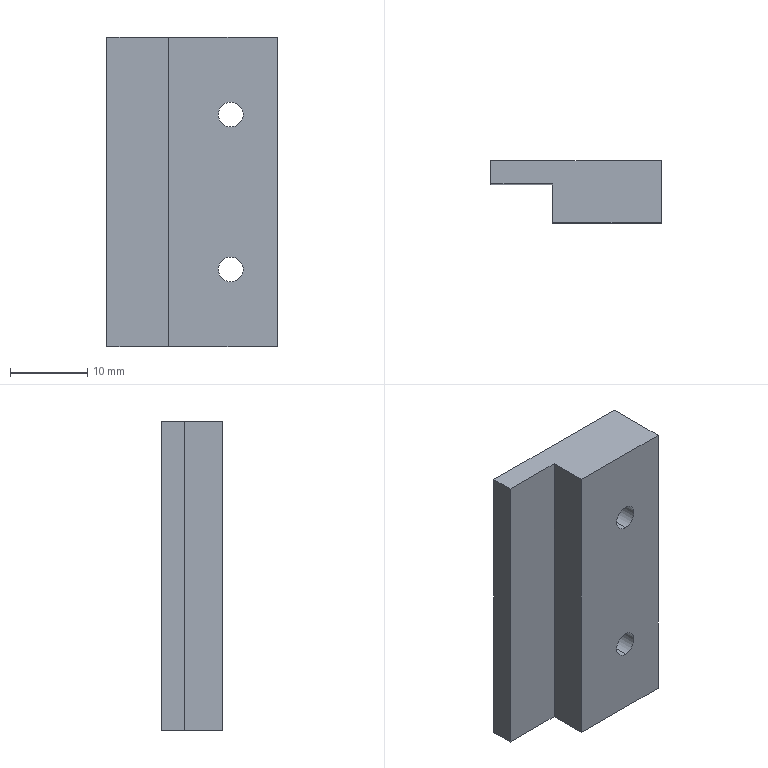Part | STEP file | PN_0053 | 1 solid | 12 faces | box 22 x 8 x 40 mm | volume 5311 mm3 | plane 8 | cylinder 4 | commonest cylinder face diameters 3.2 x4
STEP:
#1=CARTESIAN_POINT('',(0.,0.,0.));
#2=DIRECTION('',(0.,0.,1.));
#3=DIRECTION('',(1.,0.,0.));
#4=AXIS2_PLACEMENT_3D('',#1,#2,#3);
#5=CARTESIAN_POINT('',(5.,0.,11.6));
#6=VERTEX_POINT('',#5);
#7=CARTESIAN_POINT('',(5.,8.,11.6));
#8=VERTEX_POINT('',#7);
#9=CARTESIAN_POINT('',(5.,8.,11.6));
#10=DIRECTION('',(0.,1.,0.));
#11=VECTOR('',#10,1.);
#12=LINE('',#9,#11);
#13=CARTESIAN_POINT('',(5.,8.,10.));
#14=DIRECTION('',(0.,1.,0.));
#15=DIRECTION('',(0.,0.,1.));
#16=AXIS2_PLACEMENT_3D('',#13,#14,#15);
#17=CYLINDRICAL_SURFACE('',#16,1.6);
#18=CARTESIAN_POINT('',(6.283,0.));
#19=DIRECTION('',(0.,1.));
#20=VECTOR('',#19,1.);
#21=LINE('',#18,#20);
#22=(GEOMETRIC_REPRESENTATION_CONTEXT(2)PARAMETRIC_REPRESENTATION_CONTEXT()REPRESENTATION_CONTEXT('',''));
#23=DEFINITIONAL_REPRESENTATION('',(#21),#22);
#24=PCURVE('',#17,#23);
#25=CARTESIAN_POINT('',(5.,8.,10.));
#26=DIRECTION('',(0.,1.,0.));
#27=DIRECTION('',(0.,0.,1.));
#28=AXIS2_PLACEMENT_3D('',#25,#26,#27);
#29=CYLINDRICAL_SURFACE('',#28,1.6);
#30=CARTESIAN_POINT('',(0.,0.));
#31=DIRECTION('',(0.,1.));
#32=VECTOR('',#31,1.);
#33=LINE('',#30,#32);
#34=(GEOMETRIC_REPRESENTATION_CONTEXT(2)PARAMETRIC_REPRESENTATION_CONTEXT()REPRESENTATION_CONTEXT('',''));
#35=DEFINITIONAL_REPRESENTATION('',(#33),#34);
#36=PCURVE('',#29,#35);
#37=SURFACE_CURVE('',#12,(#24,#36),.PCURVE_S1.);
#38=EDGE_CURVE('',#6,#8,#37,.T.);
#39=ORIENTED_EDGE('',*,*,#38,.T.);
#40=CARTESIAN_POINT('',(5.,8.,8.4));
#41=VERTEX_POINT('',#40);
#42=CARTESIAN_POINT('',(5.,8.,10.));
#43=DIRECTION('',(0.,1.,0.));
#44=DIRECTION('',(0.,0.,1.));
#45=AXIS2_PLACEMENT_3D('',#42,#43,#44);
#46=CIRCLE('',#45,1.6);
#47=CARTESIAN_POINT('',(0.,0.));
#48=DIRECTION('',(1.,0.));
#49=VECTOR('',#48,1.);
#50=LINE('',#47,#49);
#51=(GEOMETRIC_REPRESENTATION_CONTEXT(2)PARAMETRIC_REPRESENTATION_CONTEXT()REPRESENTATION_CONTEXT('',''));
#52=DEFINITIONAL_REPRESENTATION('',(#50),#51);
#53=PCURVE('',#17,#52);
#54=CARTESIAN_POINT('',(0.,8.,0.));
#55=DIRECTION('',(0.,1.,0.));
#56=DIRECTION('',(0.,0.,1.));
#57=AXIS2_PLACEMENT_3D('',#54,#55,#56);
#58=PLANE('',#57);
#59=CARTESIAN_POINT('',(10.,5.));
#60=DIRECTION('',(1.,0.));
#61=AXIS2_PLACEMENT_2D('',#59,#60);
#62=CIRCLE('',#61,1.6);
#63=(GEOMETRIC_REPRESENTATION_CONTEXT(2)PARAMETRIC_REPRESENTATION_CONTEXT()REPRESENTATION_CONTEXT('',''));
#64=DEFINITIONAL_REPRESENTATION('',(#62),#63);
#65=PCURVE('',#58,#64);
#66=SURFACE_CURVE('',#46,(#53,#65),.PCURVE_S1.);
#67=EDGE_CURVE('',#41,#8,#66,.T.);
#68=ORIENTED_EDGE('',*,*,#67,.F.);
#69=CARTESIAN_POINT('',(5.,0.,8.4));
#70=VERTEX_POINT('',#69);
#71=CARTESIAN_POINT('',(5.,8.,8.4));
#72=DIRECTION('',(0.,1.,0.));
#73=VECTOR('',#72,1.);
#74=LINE('',#71,#73);
#75=CARTESIAN_POINT('',(3.142,0.));
#76=DIRECTION('',(0.,1.));
#77=VECTOR('',#76,1.);
#78=LINE('',#75,#77);
#79=(GEOMETRIC_REPRESENTATION_CONTEXT(2)PARAMETRIC_REPRESENTATION_CONTEXT()REPRESENTATION_CONTEXT('',''));
#80=DEFINITIONAL_REPRESENTATION('',(#78),#79);
#81=PCURVE('',#17,#80);
#82=CARTESIAN_POINT('',(3.142,0.));
#83=DIRECTION('',(0.,1.));
#84=VECTOR('',#83,1.);
#85=LINE('',#82,#84);
#86=(GEOMETRIC_REPRESENTATION_CONTEXT(2)PARAMETRIC_REPRESENTATION_CONTEXT()REPRESENTATION_CONTEXT('',''));
#87=DEFINITIONAL_REPRESENTATION('',(#85),#86);
#88=PCURVE('',#29,#87);
#89=SURFACE_CURVE('',#74,(#81,#88),.PCURVE_S1.);
#90=EDGE_CURVE('',#70,#41,#89,.T.);
#91=ORIENTED_EDGE('',*,*,#90,.F.);
#92=CARTESIAN_POINT('',(5.,0.,10.));
#93=DIRECTION('',(0.,1.,0.));
#94=DIRECTION('',(0.,0.,1.));
#95=AXIS2_PLACEMENT_3D('',#92,#93,#94);
#96=CIRCLE('',#95,1.6);
#97=CARTESIAN_POINT('',(0.,-8.));
#98=DIRECTION('',(1.,0.));
#99=VECTOR('',#98,1.);
#100=LINE('',#97,#99);
#101=(GEOMETRIC_REPRESENTATION_CONTEXT(2)PARAMETRIC_REPRESENTATION_CONTEXT()REPRESENTATION_CONTEXT('',''));
#102=DEFINITIONAL_REPRESENTATION('',(#100),#101);
#103=PCURVE('',#17,#102);
#104=CARTESIAN_POINT('',(0.,0.,0.));
#105=DIRECTION('',(0.,1.,0.));
#106=DIRECTION('',(0.,0.,1.));
#107=AXIS2_PLACEMENT_3D('',#104,#105,#106);
#108=PLANE('',#107);
#109=CARTESIAN_POINT('',(10.,5.));
#110=DIRECTION('',(1.,0.));
#111=AXIS2_PLACEMENT_2D('',#109,#110);
#112=CIRCLE('',#111,1.6);
#113=(GEOMETRIC_REPRESENTATION_CONTEXT(2)PARAMETRIC_REPRESENTATION_CONTEXT()REPRESENTATION_CONTEXT('',''));
#114=DEFINITIONAL_REPRESENTATION('',(#112),#113);
#115=PCURVE('',#108,#114);
#116=SURFACE_CURVE('',#96,(#103,#115),.PCURVE_S1.);
#117=EDGE_CURVE('',#70,#6,#116,.T.);
#118=ORIENTED_EDGE('',*,*,#117,.T.);
#119=EDGE_LOOP('',(#39,#68,#91,#118));
#120=FACE_BOUND('',#119,.F.);
#121=ADVANCED_FACE('',(#120),#17,.F.);
#122=CARTESIAN_POINT('',(5.,0.,-8.4));
#123=VERTEX_POINT('',#122);
#124=CARTESIAN_POINT('',(5.,8.,-8.4));
#125=VERTEX_POINT('',#124);
#126=CARTESIAN_POINT('',(5.,8.,-8.4));
#127=DIRECTION('',(0.,1.,0.));
#128=VECTOR('',#127,1.);
#129=LINE('',#126,#128);
#130=CARTESIAN_POINT('',(5.,8.,-10.));
#131=DIRECTION('',(0.,1.,0.));
#132=DIRECTION('',(0.,0.,1.));
#133=AXIS2_PLACEMENT_3D('',#130,#131,#132);
#134=CYLINDRICAL_SURFACE('',#133,1.6);
#135=CARTESIAN_POINT('',(6.283,0.));
#136=DIRECTION('',(0.,1.));
#137=VECTOR('',#136,1.);
#138=LINE('',#135,#137);
#139=(GEOMETRIC_REPRESENTATION_CONTEXT(2)PARAMETRIC_REPRESENTATION_CONTEXT()REPRESENTATION_CONTEXT('',''));
#140=DEFINITIONAL_REPRESENTATION('',(#138),#139);
#141=PCURVE('',#134,#140);
#142=CARTESIAN_POINT('',(5.,8.,-10.));
#143=DIRECTION('',(0.,1.,0.));
#144=DIRECTION('',(0.,0.,1.));
#145=AXIS2_PLACEMENT_3D('',#142,#143,#144);
#146=CYLINDRICAL_SURFACE('',#145,1.6);
#147=CARTESIAN_POINT('',(0.,0.));
#148=DIRECTION('',(0.,1.));
#149=VECTOR('',#148,1.);
#150=LINE('',#147,#149);
#151=(GEOMETRIC_REPRESENTATION_CONTEXT(2)PARAMETRIC_REPRESENTATION_CONTEXT()REPRESENTATION_CONTEXT('',''));
#152=DEFINITIONAL_REPRESENTATION('',(#150),#151);
#153=PCURVE('',#146,#152);
#154=SURFACE_CURVE('',#129,(#141,#153),.PCURVE_S1.);
#155=EDGE_CURVE('',#123,#125,#154,.T.);
#156=ORIENTED_EDGE('',*,*,#155,.T.);
#157=CARTESIAN_POINT('',(5.,8.,-11.6));
#158=VERTEX_POINT('',#157);
#159=CARTESIAN_POINT('',(5.,8.,-10.));
#160=DIRECTION('',(0.,1.,0.));
#161=DIRECTION('',(0.,0.,1.));
#162=AXIS2_PLACEMENT_3D('',#159,#160,#161);
#163=CIRCLE('',#162,1.6);
#164=CARTESIAN_POINT('',(0.,0.));
#165=DIRECTION('',(1.,0.));
#166=VECTOR('',#165,1.);
#167=LINE('',#164,#166);
#168=(GEOMETRIC_REPRESENTATION_CONTEXT(2)PARAMETRIC_REPRESENTATION_CONTEXT()REPRESENTATION_CONTEXT('',''));
#169=DEFINITIONAL_REPRESENTATION('',(#167),#168);
#170=PCURVE('',#134,#169);
#171=CARTESIAN_POINT('',(-10.,5.));
#172=DIRECTION('',(1.,0.));
#173=AXIS2_PLACEMENT_2D('',#171,#172);
#174=CIRCLE('',#173,1.6);
#175=(GEOMETRIC_REPRESENTATION_CONTEXT(2)PARAMETRIC_REPRESENTATION_CONTEXT()REPRESENTATION_CONTEXT('',''));
#176=DEFINITIONAL_REPRESENTATION('',(#174),#175);
#177=PCURVE('',#58,#176);
#178=SURFACE_CURVE('',#163,(#170,#177),.PCURVE_S1.);
#179=EDGE_CURVE('',#158,#125,#178,.T.);
#180=ORIENTED_EDGE('',*,*,#179,.F.);
#181=CARTESIAN_POINT('',(5.,0.,-11.6));
#182=VERTEX_POINT('',#181);
#183=CARTESIAN_POINT('',(5.,8.,-11.6));
#184=DIRECTION('',(0.,1.,0.));
#185=VECTOR('',#184,1.);
#186=LINE('',#183,#185);
#187=CARTESIAN_POINT('',(3.142,0.));
#188=DIRECTION('',(0.,1.));
#189=VECTOR('',#188,1.);
#190=LINE('',#187,#189);
#191=(GEOMETRIC_REPRESENTATION_CONTEXT(2)PARAMETRIC_REPRESENTATION_CONTEXT()REPRESENTATION_CONTEXT('',''));
#192=DEFINITIONAL_REPRESENTATION('',(#190),#191);
#193=PCURVE('',#134,#192);
#194=CARTESIAN_POINT('',(3.142,0.));
#195=DIRECTION('',(0.,1.));
#196=VECTOR('',#195,1.);
#197=LINE('',#194,#196);
#198=(GEOMETRIC_REPRESENTATION_CONTEXT(2)PARAMETRIC_REPRESENTATION_CONTEXT()REPRESENTATION_CONTEXT('',''));
#199=DEFINITIONAL_REPRESENTATION('',(#197),#198);
#200=PCURVE('',#146,#199);
#201=SURFACE_CURVE('',#186,(#193,#200),.PCURVE_S1.);
#202=EDGE_CURVE('',#182,#158,#201,.T.);
#203=ORIENTED_EDGE('',*,*,#202,.F.);
#204=CARTESIAN_POINT('',(5.,0.,-10.));
#205=DIRECTION('',(0.,1.,0.));
#206=DIRECTION('',(0.,0.,1.));
#207=AXIS2_PLACEMENT_3D('',#204,#205,#206);
#208=CIRCLE('',#207,1.6);
#209=CARTESIAN_POINT('',(0.,-8.));
#210=DIRECTION('',(1.,0.));
#211=VECTOR('',#210,1.);
#212=LINE('',#209,#211);
#213=(GEOMETRIC_REPRESENTATION_CONTEXT(2)PARAMETRIC_REPRESENTATION_CONTEXT()REPRESENTATION_CONTEXT('',''));
#214=DEFINITIONAL_REPRESENTATION('',(#212),#213);
#215=PCURVE('',#134,#214);
#216=CARTESIAN_POINT('',(-10.,5.));
#217=DIRECTION('',(1.,0.));
#218=AXIS2_PLACEMENT_2D('',#216,#217);
#219=CIRCLE('',#218,1.6);
#220=(GEOMETRIC_REPRESENTATION_CONTEXT(2)PARAMETRIC_REPRESENTATION_CONTEXT()REPRESENTATION_CONTEXT('',''));
#221=DEFINITIONAL_REPRESENTATION('',(#219),#220);
#222=PCURVE('',#108,#221);
#223=SURFACE_CURVE('',#208,(#215,#222),.PCURVE_S1.);
#224=EDGE_CURVE('',#182,#123,#223,.T.);
#225=ORIENTED_EDGE('',*,*,#224,.T.);
#226=EDGE_LOOP('',(#156,#180,#203,#225));
#227=FACE_BOUND('',#226,.F.);
#228=ADVANCED_FACE('',(#227),#134,.F.);
#229=CARTESIAN_POINT('',(11.,0.,20.));
#230=VERTEX_POINT('',#229);
#231=CARTESIAN_POINT('',(11.,0.,-20.));
#232=VERTEX_POINT('',#231);
#233=CARTESIAN_POINT('',(11.,0.,-20.));
#234=DIRECTION('',(0.,0.,-1.));
#235=VECTOR('',#234,1.);
#236=LINE('',#233,#235);
#237=CARTESIAN_POINT('',(11.,8.,-20.));
#238=DIRECTION('',(-1.,0.,0.));
#239=DIRECTION('',(0.,0.,1.));
#240=AXIS2_PLACEMENT_3D('',#237,#238,#239);
#241=PLANE('',#240);
#242=CARTESIAN_POINT('',(0.,-8.));
#243=DIRECTION('',(-1.,0.));
#244=VECTOR('',#243,1.);
#245=LINE('',#242,#244);
#246=(GEOMETRIC_REPRESENTATION_CONTEXT(2)PARAMETRIC_REPRESENTATION_CONTEXT()REPRESENTATION_CONTEXT('',''));
#247=DEFINITIONAL_REPRESENTATION('',(#245),#246);
#248=PCURVE('',#241,#247);
#249=CARTESIAN_POINT('',(-20.,11.));
#250=DIRECTION('',(-1.,0.));
#251=VECTOR('',#250,1.);
#252=LINE('',#249,#251);
#253=(GEOMETRIC_REPRESENTATION_CONTEXT(2)PARAMETRIC_REPRESENTATION_CONTEXT()REPRESENTATION_CONTEXT('',''));
#254=DEFINITIONAL_REPRESENTATION('',(#252),#253);
#255=PCURVE('',#108,#254);
#256=SURFACE_CURVE('',#236,(#248,#255),.PCURVE_S1.);
#257=EDGE_CURVE('',#230,#232,#256,.T.);
#258=ORIENTED_EDGE('',*,*,#257,.T.);
#259=CARTESIAN_POINT('',(11.,8.,-20.));
#260=VERTEX_POINT('',#259);
#261=CARTESIAN_POINT('',(11.,8.,-20.));
#262=DIRECTION('',(0.,-1.,0.));
#263=VECTOR('',#262,1.);
#264=LINE('',#261,#263);
#265=CARTESIAN_POINT('',(0.,0.));
#266=DIRECTION('',(0.,-1.));
#267=VECTOR('',#266,1.);
#268=LINE('',#265,#267);
#269=(GEOMETRIC_REPRESENTATION_CONTEXT(2)PARAMETRIC_REPRESENTATION_CONTEXT()REPRESENTATION_CONTEXT('',''));
#270=DEFINITIONAL_REPRESENTATION('',(#268),#269);
#271=PCURVE('',#241,#270);
#272=CARTESIAN_POINT('',(-11.,8.,-20.));
#273=DIRECTION('',(0.,0.,1.));
#274=DIRECTION('',(1.,0.,0.));
#275=AXIS2_PLACEMENT_3D('',#272,#273,#274);
#276=PLANE('',#275);
#277=CARTESIAN_POINT('',(22.,0.));
#278=DIRECTION('',(0.,-1.));
#279=VECTOR('',#278,1.);
#280=LINE('',#277,#279);
#281=(GEOMETRIC_REPRESENTATION_CONTEXT(2)PARAMETRIC_REPRESENTATION_CONTEXT()REPRESENTATION_CONTEXT('',''));
#282=DEFINITIONAL_REPRESENTATION('',(#280),#281);
#283=PCURVE('',#276,#282);
#284=SURFACE_CURVE('',#264,(#271,#283),.PCURVE_S1.);
#285=EDGE_CURVE('',#260,#232,#284,.T.);
#286=ORIENTED_EDGE('',*,*,#285,.F.);
#287=CARTESIAN_POINT('',(11.,8.,20.));
#288=VERTEX_POINT('',#287);
#289=CARTESIAN_POINT('',(11.,8.,-20.));
#290=DIRECTION('',(0.,0.,-1.));
#291=VECTOR('',#290,1.);
#292=LINE('',#289,#291);
#293=CARTESIAN_POINT('',(0.,0.));
#294=DIRECTION('',(-1.,0.));
#295=VECTOR('',#294,1.);
#296=LINE('',#293,#295);
#297=(GEOMETRIC_REPRESENTATION_CONTEXT(2)PARAMETRIC_REPRESENTATION_CONTEXT()REPRESENTATION_CONTEXT('',''));
#298=DEFINITIONAL_REPRESENTATION('',(#296),#297);
#299=PCURVE('',#241,#298);
#300=CARTESIAN_POINT('',(-20.,11.));
#301=DIRECTION('',(-1.,0.));
#302=VECTOR('',#301,1.);
#303=LINE('',#300,#302);
#304=(GEOMETRIC_REPRESENTATION_CONTEXT(2)PARAMETRIC_REPRESENTATION_CONTEXT()REPRESENTATION_CONTEXT('',''));
#305=DEFINITIONAL_REPRESENTATION('',(#303),#304);
#306=PCURVE('',#58,#305);
#307=SURFACE_CURVE('',#292,(#299,#306),.PCURVE_S1.);
#308=EDGE_CURVE('',#288,#260,#307,.T.);
#309=ORIENTED_EDGE('',*,*,#308,.F.);
#310=CARTESIAN_POINT('',(11.,8.,20.));
#311=DIRECTION('',(0.,-1.,0.));
#312=VECTOR('',#311,1.);
#313=LINE('',#310,#312);
#314=CARTESIAN_POINT('',(40.,0.));
#315=DIRECTION('',(0.,-1.));
#316=VECTOR('',#315,1.);
#317=LINE('',#314,#316);
#318=(GEOMETRIC_REPRESENTATION_CONTEXT(2)PARAMETRIC_REPRESENTATION_CONTEXT()REPRESENTATION_CONTEXT('',''));
#319=DEFINITIONAL_REPRESENTATION('',(#317),#318);
#320=PCURVE('',#241,#319);
#321=CARTESIAN_POINT('',(-11.,8.,20.));
#322=DIRECTION('',(0.,0.,-1.));
#323=DIRECTION('',(-1.,0.,0.));
#324=AXIS2_PLACEMENT_3D('',#321,#322,#323);
#325=PLANE('',#324);
#326=CARTESIAN_POINT('',(-22.,0.));
#327=DIRECTION('',(0.,-1.));
#328=VECTOR('',#327,1.);
#329=LINE('',#326,#328);
#330=(GEOMETRIC_REPRESENTATION_CONTEXT(2)PARAMETRIC_REPRESENTATION_CONTEXT()REPRESENTATION_CONTEXT('',''));
#331=DEFINITIONAL_REPRESENTATION('',(#329),#330);
#332=PCURVE('',#325,#331);
#333=SURFACE_CURVE('',#313,(#320,#332),.PCURVE_S1.);
#334=EDGE_CURVE('',#288,#230,#333,.T.);
#335=ORIENTED_EDGE('',*,*,#334,.T.);
#336=EDGE_LOOP('',(#258,#286,#309,#335));
#337=FACE_BOUND('',#336,.T.);
#338=ADVANCED_FACE('',(#337),#241,.F.);
#339=CARTESIAN_POINT('',(-3.,0.,-20.));
#340=VERTEX_POINT('',#339);
#341=CARTESIAN_POINT('',(-3.,5.,-20.));
#342=VERTEX_POINT('',#341);
#343=CARTESIAN_POINT('',(-3.,0.,-20.));
#344=DIRECTION('',(0.,1.,0.));
#345=VECTOR('',#344,1.);
#346=LINE('',#343,#345);
#347=CARTESIAN_POINT('',(8.,-8.));
#348=DIRECTION('',(0.,1.));
#349=VECTOR('',#348,1.);
#350=LINE('',#347,#349);
#351=(GEOMETRIC_REPRESENTATION_CONTEXT(2)PARAMETRIC_REPRESENTATION_CONTEXT()REPRESENTATION_CONTEXT('',''));
#352=DEFINITIONAL_REPRESENTATION('',(#350),#351);
#353=PCURVE('',#276,#352);
#354=CARTESIAN_POINT('',(-3.,0.,-20.));
#355=DIRECTION('',(1.,0.,0.));
#356=DIRECTION('',(0.,0.,-1.));
#357=AXIS2_PLACEMENT_3D('',#354,#355,#356);
#358=PLANE('',#357);
#359=CARTESIAN_POINT('',(0.,0.));
#360=DIRECTION('',(0.,1.));
#361=VECTOR('',#360,1.);
#362=LINE('',#359,#361);
#363=(GEOMETRIC_REPRESENTATION_CONTEXT(2)PARAMETRIC_REPRESENTATION_CONTEXT()REPRESENTATION_CONTEXT('',''));
#364=DEFINITIONAL_REPRESENTATION('',(#362),#363);
#365=PCURVE('',#358,#364);
#366=SURFACE_CURVE('',#346,(#353,#365),.PCURVE_S1.);
#367=EDGE_CURVE('',#340,#342,#366,.T.);
#368=ORIENTED_EDGE('',*,*,#367,.T.);
#369=CARTESIAN_POINT('',(-11.,5.,-20.));
#370=VERTEX_POINT('',#369);
#371=CARTESIAN_POINT('',(-11.,5.,-20.));
#372=DIRECTION('',(-1.,0.,0.));
#373=VECTOR('',#372,1.);
#374=LINE('',#371,#373);
#375=CARTESIAN_POINT('',(0.,-3.));
#376=DIRECTION('',(-1.,0.));
#377=VECTOR('',#376,1.);
#378=LINE('',#375,#377);
#379=(GEOMETRIC_REPRESENTATION_CONTEXT(2)PARAMETRIC_REPRESENTATION_CONTEXT()REPRESENTATION_CONTEXT('',''));
#380=DEFINITIONAL_REPRESENTATION('',(#378),#379);
#381=PCURVE('',#276,#380);
#382=CARTESIAN_POINT('',(-11.,5.,-20.));
#383=DIRECTION('',(0.,1.,0.));
#384=DIRECTION('',(0.,0.,1.));
#385=AXIS2_PLACEMENT_3D('',#382,#383,#384);
#386=PLANE('',#385);
#387=CARTESIAN_POINT('',(0.,0.));
#388=DIRECTION('',(0.,-1.));
#389=VECTOR('',#388,1.);
#390=LINE('',#387,#389);
#391=(GEOMETRIC_REPRESENTATION_CONTEXT(2)PARAMETRIC_REPRESENTATION_CONTEXT()REPRESENTATION_CONTEXT('',''));
#392=DEFINITIONAL_REPRESENTATION('',(#390),#391);
#393=PCURVE('',#386,#392);
#394=SURFACE_CURVE('',#374,(#381,#393),.PCURVE_S1.);
#395=EDGE_CURVE('',#342,#370,#394,.T.);
#396=ORIENTED_EDGE('',*,*,#395,.T.);
#397=CARTESIAN_POINT('',(-11.,8.,-20.));
#398=VERTEX_POINT('',#397);
#399=CARTESIAN_POINT('',(-11.,8.,-20.));
#400=DIRECTION('',(0.,-1.,0.));
#401=VECTOR('',#400,1.);
#402=LINE('',#399,#401);
#403=CARTESIAN_POINT('',(0.,0.));
#404=DIRECTION('',(0.,-1.));
#405=VECTOR('',#404,1.);
#406=LINE('',#403,#405);
#407=(GEOMETRIC_REPRESENTATION_CONTEXT(2)PARAMETRIC_REPRESENTATION_CONTEXT()REPRESENTATION_CONTEXT('',''));
#408=DEFINITIONAL_REPRESENTATION('',(#406),#407);
#409=PCURVE('',#276,#408);
#410=CARTESIAN_POINT('',(-11.,8.,-20.));
#411=DIRECTION('',(1.,0.,0.));
#412=DIRECTION('',(0.,0.,-1.));
#413=AXIS2_PLACEMENT_3D('',#410,#411,#412);
#414=PLANE('',#413);
#415=CARTESIAN_POINT('',(0.,0.));
#416=DIRECTION('',(0.,-1.));
#417=VECTOR('',#416,1.);
#418=LINE('',#415,#417);
#419=(GEOMETRIC_REPRESENTATION_CONTEXT(2)PARAMETRIC_REPRESENTATION_CONTEXT()REPRESENTATION_CONTEXT('',''));
#420=DEFINITIONAL_REPRESENTATION('',(#418),#419);
#421=PCURVE('',#414,#420);
#422=SURFACE_CURVE('',#402,(#409,#421),.PCURVE_S1.);
#423=EDGE_CURVE('',#398,#370,#422,.T.);
#424=ORIENTED_EDGE('',*,*,#423,.F.);
#425=CARTESIAN_POINT('',(-11.,8.,-20.));
#426=DIRECTION('',(-1.,0.,0.));
#427=VECTOR('',#426,1.);
#428=LINE('',#425,#427);
#429=CARTESIAN_POINT('',(0.,0.));
#430=DIRECTION('',(-1.,0.));
#431=VECTOR('',#430,1.);
#432=LINE('',#429,#431);
#433=(GEOMETRIC_REPRESENTATION_CONTEXT(2)PARAMETRIC_REPRESENTATION_CONTEXT()REPRESENTATION_CONTEXT('',''));
#434=DEFINITIONAL_REPRESENTATION('',(#432),#433);
#435=PCURVE('',#276,#434);
#436=CARTESIAN_POINT('',(-20.,-11.));
#437=DIRECTION('',(0.,-1.));
#438=VECTOR('',#437,1.);
#439=LINE('',#436,#438);
#440=(GEOMETRIC_REPRESENTATION_CONTEXT(2)PARAMETRIC_REPRESENTATION_CONTEXT()REPRESENTATION_CONTEXT('',''));
#441=DEFINITIONAL_REPRESENTATION('',(#439),#440);
#442=PCURVE('',#58,#441);
#443=SURFACE_CURVE('',#428,(#435,#442),.PCURVE_S1.);
#444=EDGE_CURVE('',#260,#398,#443,.T.);
#445=ORIENTED_EDGE('',*,*,#444,.F.);
#446=ORIENTED_EDGE('',*,*,#285,.T.);
#447=CARTESIAN_POINT('',(-11.,0.,-20.));
#448=DIRECTION('',(-1.,0.,0.));
#449=VECTOR('',#448,1.);
#450=LINE('',#447,#449);
#451=CARTESIAN_POINT('',(0.,-8.));
#452=DIRECTION('',(-1.,0.));
#453=VECTOR('',#452,1.);
#454=LINE('',#451,#453);
#455=(GEOMETRIC_REPRESENTATION_CONTEXT(2)PARAMETRIC_REPRESENTATION_CONTEXT()REPRESENTATION_CONTEXT('',''));
#456=DEFINITIONAL_REPRESENTATION('',(#454),#455);
#457=PCURVE('',#276,#456);
#458=CARTESIAN_POINT('',(-20.,-11.));
#459=DIRECTION('',(0.,-1.));
#460=VECTOR('',#459,1.);
#461=LINE('',#458,#460);
#462=(GEOMETRIC_REPRESENTATION_CONTEXT(2)PARAMETRIC_REPRESENTATION_CONTEXT()REPRESENTATION_CONTEXT('',''));
#463=DEFINITIONAL_REPRESENTATION('',(#461),#462);
#464=PCURVE('',#108,#463);
#465=SURFACE_CURVE('',#450,(#457,#464),.PCURVE_S1.);
#466=EDGE_CURVE('',#232,#340,#465,.T.);
#467=ORIENTED_EDGE('',*,*,#466,.T.);
#468=EDGE_LOOP('',(#368,#396,#424,#445,#446,#467));
#469=FACE_BOUND('',#468,.T.);
#470=ADVANCED_FACE('',(#469),#276,.F.);
#471=ORIENTED_EDGE('',*,*,#423,.T.);
#472=CARTESIAN_POINT('',(-11.,5.,20.));
#473=VERTEX_POINT('',#472);
#474=CARTESIAN_POINT('',(-11.,5.,-20.));
#475=DIRECTION('',(0.,0.,1.));
#476=VECTOR('',#475,1.);
#477=LINE('',#474,#476);
#478=CARTESIAN_POINT('',(0.,-3.));
#479=DIRECTION('',(-1.,0.));
#480=VECTOR('',#479,1.);
#481=LINE('',#478,#480);
#482=(GEOMETRIC_REPRESENTATION_CONTEXT(2)PARAMETRIC_REPRESENTATION_CONTEXT()REPRESENTATION_CONTEXT('',''));
#483=DEFINITIONAL_REPRESENTATION('',(#481),#482);
#484=PCURVE('',#414,#483);
#485=CARTESIAN_POINT('',(0.,0.));
#486=DIRECTION('',(1.,0.));
#487=VECTOR('',#486,1.);
#488=LINE('',#485,#487);
#489=(GEOMETRIC_REPRESENTATION_CONTEXT(2)PARAMETRIC_REPRESENTATION_CONTEXT()REPRESENTATION_CONTEXT('',''));
#490=DEFINITIONAL_REPRESENTATION('',(#488),#489);
#491=PCURVE('',#386,#490);
#492=SURFACE_CURVE('',#477,(#484,#491),.PCURVE_S1.);
#493=EDGE_CURVE('',#370,#473,#492,.T.);
#494=ORIENTED_EDGE('',*,*,#493,.T.);
#495=CARTESIAN_POINT('',(-11.,8.,20.));
#496=VERTEX_POINT('',#495);
#497=CARTESIAN_POINT('',(-11.,8.,20.));
#498=DIRECTION('',(0.,-1.,0.));
#499=VECTOR('',#498,1.);
#500=LINE('',#497,#499);
#501=CARTESIAN_POINT('',(-40.,0.));
#502=DIRECTION('',(0.,-1.));
#503=VECTOR('',#502,1.);
#504=LINE('',#501,#503);
#505=(GEOMETRIC_REPRESENTATION_CONTEXT(2)PARAMETRIC_REPRESENTATION_CONTEXT()REPRESENTATION_CONTEXT('',''));
#506=DEFINITIONAL_REPRESENTATION('',(#504),#505);
#507=PCURVE('',#414,#506);
#508=CARTESIAN_POINT('',(0.,0.));
#509=DIRECTION('',(0.,-1.));
#510=VECTOR('',#509,1.);
#511=LINE('',#508,#510);
#512=(GEOMETRIC_REPRESENTATION_CONTEXT(2)PARAMETRIC_REPRESENTATION_CONTEXT()REPRESENTATION_CONTEXT('',''));
#513=DEFINITIONAL_REPRESENTATION('',(#511),#512);
#514=PCURVE('',#325,#513);
#515=SURFACE_CURVE('',#500,(#507,#514),.PCURVE_S1.);
#516=EDGE_CURVE('',#496,#473,#515,.T.);
#517=ORIENTED_EDGE('',*,*,#516,.F.);
#518=CARTESIAN_POINT('',(-11.,8.,-20.));
#519=DIRECTION('',(0.,0.,1.));
#520=VECTOR('',#519,1.);
#521=LINE('',#518,#520);
#522=CARTESIAN_POINT('',(0.,0.));
#523=DIRECTION('',(-1.,0.));
#524=VECTOR('',#523,1.);
#525=LINE('',#522,#524);
#526=(GEOMETRIC_REPRESENTATION_CONTEXT(2)PARAMETRIC_REPRESENTATION_CONTEXT()REPRESENTATION_CONTEXT('',''));
#527=DEFINITIONAL_REPRESENTATION('',(#525),#526);
#528=PCURVE('',#414,#527);
#529=CARTESIAN_POINT('',(-20.,-11.));
#530=DIRECTION('',(1.,0.));
#531=VECTOR('',#530,1.);
#532=LINE('',#529,#531);
#533=(GEOMETRIC_REPRESENTATION_CONTEXT(2)PARAMETRIC_REPRESENTATION_CONTEXT()REPRESENTATION_CONTEXT('',''));
#534=DEFINITIONAL_REPRESENTATION('',(#532),#533);
#535=PCURVE('',#58,#534);
#536=SURFACE_CURVE('',#521,(#528,#535),.PCURVE_S1.);
#537=EDGE_CURVE('',#398,#496,#536,.T.);
#538=ORIENTED_EDGE('',*,*,#537,.F.);
#539=EDGE_LOOP('',(#471,#494,#517,#538));
#540=FACE_BOUND('',#539,.T.);
#541=ADVANCED_FACE('',(#540),#414,.F.);
#542=ORIENTED_EDGE('',*,*,#516,.T.);
#543=CARTESIAN_POINT('',(-3.,5.,20.));
#544=VERTEX_POINT('',#543);
#545=CARTESIAN_POINT('',(-11.,5.,20.));
#546=DIRECTION('',(-1.,0.,0.));
#547=VECTOR('',#546,1.);
#548=LINE('',#545,#547);
#549=CARTESIAN_POINT('',(0.,-3.));
#550=DIRECTION('',(1.,0.));
#551=VECTOR('',#550,1.);
#552=LINE('',#549,#551);
#553=(GEOMETRIC_REPRESENTATION_CONTEXT(2)PARAMETRIC_REPRESENTATION_CONTEXT()REPRESENTATION_CONTEXT('',''));
#554=DEFINITIONAL_REPRESENTATION('',(#552),#553);
#555=PCURVE('',#325,#554);
#556=CARTESIAN_POINT('',(40.,0.));
#557=DIRECTION('',(0.,-1.));
#558=VECTOR('',#557,1.);
#559=LINE('',#556,#558);
#560=(GEOMETRIC_REPRESENTATION_CONTEXT(2)PARAMETRIC_REPRESENTATION_CONTEXT()REPRESENTATION_CONTEXT('',''));
#561=DEFINITIONAL_REPRESENTATION('',(#559),#560);
#562=PCURVE('',#386,#561);
#563=SURFACE_CURVE('',#548,(#555,#562),.PCURVE_S1.);
#564=EDGE_CURVE('',#544,#473,#563,.T.);
#565=ORIENTED_EDGE('',*,*,#564,.F.);
#566=CARTESIAN_POINT('',(-3.,0.,20.));
#567=VERTEX_POINT('',#566);
#568=CARTESIAN_POINT('',(-3.,0.,20.));
#569=DIRECTION('',(0.,1.,0.));
#570=VECTOR('',#569,1.);
#571=LINE('',#568,#570);
#572=CARTESIAN_POINT('',(-8.,-8.));
#573=DIRECTION('',(0.,1.));
#574=VECTOR('',#573,1.);
#575=LINE('',#572,#574);
#576=(GEOMETRIC_REPRESENTATION_CONTEXT(2)PARAMETRIC_REPRESENTATION_CONTEXT()REPRESENTATION_CONTEXT('',''));
#577=DEFINITIONAL_REPRESENTATION('',(#575),#576);
#578=PCURVE('',#325,#577);
#579=CARTESIAN_POINT('',(-40.,0.));
#580=DIRECTION('',(0.,1.));
#581=VECTOR('',#580,1.);
#582=LINE('',#579,#581);
#583=(GEOMETRIC_REPRESENTATION_CONTEXT(2)PARAMETRIC_REPRESENTATION_CONTEXT()REPRESENTATION_CONTEXT('',''));
#584=DEFINITIONAL_REPRESENTATION('',(#582),#583);
#585=PCURVE('',#358,#584);
#586=SURFACE_CURVE('',#571,(#578,#585),.PCURVE_S1.);
#587=EDGE_CURVE('',#567,#544,#586,.T.);
#588=ORIENTED_EDGE('',*,*,#587,.F.);
#589=CARTESIAN_POINT('',(-11.,0.,20.));
#590=DIRECTION('',(1.,0.,0.));
#591=VECTOR('',#590,1.);
#592=LINE('',#589,#591);
#593=CARTESIAN_POINT('',(0.,-8.));
#594=DIRECTION('',(-1.,0.));
#595=VECTOR('',#594,1.);
#596=LINE('',#593,#595);
#597=(GEOMETRIC_REPRESENTATION_CONTEXT(2)PARAMETRIC_REPRESENTATION_CONTEXT()REPRESENTATION_CONTEXT('',''));
#598=DEFINITIONAL_REPRESENTATION('',(#596),#597);
#599=PCURVE('',#325,#598);
#600=CARTESIAN_POINT('',(20.,-11.));
#601=DIRECTION('',(0.,1.));
#602=VECTOR('',#601,1.);
#603=LINE('',#600,#602);
#604=(GEOMETRIC_REPRESENTATION_CONTEXT(2)PARAMETRIC_REPRESENTATION_CONTEXT()REPRESENTATION_CONTEXT('',''));
#605=DEFINITIONAL_REPRESENTATION('',(#603),#604);
#606=PCURVE('',#108,#605);
#607=SURFACE_CURVE('',#592,(#599,#606),.PCURVE_S1.);
#608=EDGE_CURVE('',#567,#230,#607,.T.);
#609=ORIENTED_EDGE('',*,*,#608,.T.);
#610=ORIENTED_EDGE('',*,*,#334,.F.);
#611=CARTESIAN_POINT('',(-11.,8.,20.));
#612=DIRECTION('',(1.,0.,0.));
#613=VECTOR('',#612,1.);
#614=LINE('',#611,#613);
#615=CARTESIAN_POINT('',(0.,0.));
#616=DIRECTION('',(-1.,0.));
#617=VECTOR('',#616,1.);
#618=LINE('',#615,#617);
#619=(GEOMETRIC_REPRESENTATION_CONTEXT(2)PARAMETRIC_REPRESENTATION_CONTEXT()REPRESENTATION_CONTEXT('',''));
#620=DEFINITIONAL_REPRESENTATION('',(#618),#619);
#621=PCURVE('',#325,#620);
#622=CARTESIAN_POINT('',(20.,-11.));
#623=DIRECTION('',(0.,1.));
#624=VECTOR('',#623,1.);
#625=LINE('',#622,#624);
#626=(GEOMETRIC_REPRESENTATION_CONTEXT(2)PARAMETRIC_REPRESENTATION_CONTEXT()REPRESENTATION_CONTEXT('',''));
#627=DEFINITIONAL_REPRESENTATION('',(#625),#626);
#628=PCURVE('',#58,#627);
#629=SURFACE_CURVE('',#614,(#621,#628),.PCURVE_S1.);
#630=EDGE_CURVE('',#496,#288,#629,.T.);
#631=ORIENTED_EDGE('',*,*,#630,.F.);
#632=EDGE_LOOP('',(#542,#565,#588,#609,#610,#631));
#633=FACE_BOUND('',#632,.T.);
#634=ADVANCED_FACE('',(#633),#325,.F.);
#635=CARTESIAN_POINT('',(5.,8.,10.));
#636=DIRECTION('',(0.,1.,0.));
#637=DIRECTION('',(0.,0.,1.));
#638=AXIS2_PLACEMENT_3D('',#635,#636,#637);
#639=CIRCLE('',#638,1.6);
#640=CARTESIAN_POINT('',(10.,5.));
#641=DIRECTION('',(1.,0.));
#642=AXIS2_PLACEMENT_2D('',#640,#641);
#643=CIRCLE('',#642,1.6);
#644=(GEOMETRIC_REPRESENTATION_CONTEXT(2)PARAMETRIC_REPRESENTATION_CONTEXT()REPRESENTATION_CONTEXT('',''));
#645=DEFINITIONAL_REPRESENTATION('',(#643),#644);
#646=PCURVE('',#58,#645);
#647=CARTESIAN_POINT('',(0.,0.));
#648=DIRECTION('',(1.,0.));
#649=VECTOR('',#648,1.);
#650=LINE('',#647,#649);
#651=(GEOMETRIC_REPRESENTATION_CONTEXT(2)PARAMETRIC_REPRESENTATION_CONTEXT()REPRESENTATION_CONTEXT('',''));
#652=DEFINITIONAL_REPRESENTATION('',(#650),#651);
#653=PCURVE('',#29,#652);
#654=SURFACE_CURVE('',#639,(#646,#653),.PCURVE_S1.);
#655=EDGE_CURVE('',#8,#41,#654,.T.);
#656=ORIENTED_EDGE('',*,*,#655,.F.);
#657=ORIENTED_EDGE('',*,*,#67,.F.);
#658=EDGE_LOOP('',(#656,#657));
#659=FACE_BOUND('',#658,.T.);
#660=CARTESIAN_POINT('',(5.,8.,-10.));
#661=DIRECTION('',(0.,1.,0.));
#662=DIRECTION('',(0.,0.,1.));
#663=AXIS2_PLACEMENT_3D('',#660,#661,#662);
#664=CIRCLE('',#663,1.6);
#665=CARTESIAN_POINT('',(-10.,5.));
#666=DIRECTION('',(1.,0.));
#667=AXIS2_PLACEMENT_2D('',#665,#666);
#668=CIRCLE('',#667,1.6);
#669=(GEOMETRIC_REPRESENTATION_CONTEXT(2)PARAMETRIC_REPRESENTATION_CONTEXT()REPRESENTATION_CONTEXT('',''));
#670=DEFINITIONAL_REPRESENTATION('',(#668),#669);
#671=PCURVE('',#58,#670);
#672=CARTESIAN_POINT('',(0.,0.));
#673=DIRECTION('',(1.,0.));
#674=VECTOR('',#673,1.);
#675=LINE('',#672,#674);
#676=(GEOMETRIC_REPRESENTATION_CONTEXT(2)PARAMETRIC_REPRESENTATION_CONTEXT()REPRESENTATION_CONTEXT('',''));
#677=DEFINITIONAL_REPRESENTATION('',(#675),#676);
#678=PCURVE('',#146,#677);
#679=SURFACE_CURVE('',#664,(#671,#678),.PCURVE_S1.);
#680=EDGE_CURVE('',#125,#158,#679,.T.);
#681=ORIENTED_EDGE('',*,*,#680,.F.);
#682=ORIENTED_EDGE('',*,*,#179,.F.);
#683=EDGE_LOOP('',(#681,#682));
#684=FACE_BOUND('',#683,.T.);
#685=ORIENTED_EDGE('',*,*,#308,.T.);
#686=ORIENTED_EDGE('',*,*,#444,.T.);
#687=ORIENTED_EDGE('',*,*,#537,.T.);
#688=ORIENTED_EDGE('',*,*,#630,.T.);
#689=EDGE_LOOP('',(#685,#686,#687,#688));
#690=FACE_BOUND('',#689,.T.);
#691=ADVANCED_FACE('',(#659,#684,#690),#58,.T.);
#692=CARTESIAN_POINT('',(5.,0.,10.));
#693=DIRECTION('',(0.,1.,0.));
#694=DIRECTION('',(0.,0.,1.));
#695=AXIS2_PLACEMENT_3D('',#692,#693,#694);
#696=CIRCLE('',#695,1.6);
#697=CARTESIAN_POINT('',(10.,5.));
#698=DIRECTION('',(1.,0.));
#699=AXIS2_PLACEMENT_2D('',#697,#698);
#700=CIRCLE('',#699,1.6);
#701=(GEOMETRIC_REPRESENTATION_CONTEXT(2)PARAMETRIC_REPRESENTATION_CONTEXT()REPRESENTATION_CONTEXT('',''));
#702=DEFINITIONAL_REPRESENTATION('',(#700),#701);
#703=PCURVE('',#108,#702);
#704=CARTESIAN_POINT('',(0.,-8.));
#705=DIRECTION('',(1.,0.));
#706=VECTOR('',#705,1.);
#707=LINE('',#704,#706);
#708=(GEOMETRIC_REPRESENTATION_CONTEXT(2)PARAMETRIC_REPRESENTATION_CONTEXT()REPRESENTATION_CONTEXT('',''));
#709=DEFINITIONAL_REPRESENTATION('',(#707),#708);
#710=PCURVE('',#29,#709);
#711=SURFACE_CURVE('',#696,(#703,#710),.PCURVE_S1.);
#712=EDGE_CURVE('',#6,#70,#711,.T.);
#713=ORIENTED_EDGE('',*,*,#712,.T.);
#714=ORIENTED_EDGE('',*,*,#117,.T.);
#715=EDGE_LOOP('',(#713,#714));
#716=FACE_BOUND('',#715,.T.);
#717=CARTESIAN_POINT('',(5.,0.,-10.));
#718=DIRECTION('',(0.,1.,0.));
#719=DIRECTION('',(0.,0.,1.));
#720=AXIS2_PLACEMENT_3D('',#717,#718,#719);
#721=CIRCLE('',#720,1.6);
#722=CARTESIAN_POINT('',(-10.,5.));
#723=DIRECTION('',(1.,0.));
#724=AXIS2_PLACEMENT_2D('',#722,#723);
#725=CIRCLE('',#724,1.6);
#726=(GEOMETRIC_REPRESENTATION_CONTEXT(2)PARAMETRIC_REPRESENTATION_CONTEXT()REPRESENTATION_CONTEXT('',''));
#727=DEFINITIONAL_REPRESENTATION('',(#725),#726);
#728=PCURVE('',#108,#727);
#729=CARTESIAN_POINT('',(0.,-8.));
#730=DIRECTION('',(1.,0.));
#731=VECTOR('',#730,1.);
#732=LINE('',#729,#731);
#733=(GEOMETRIC_REPRESENTATION_CONTEXT(2)PARAMETRIC_REPRESENTATION_CONTEXT()REPRESENTATION_CONTEXT('',''));
#734=DEFINITIONAL_REPRESENTATION('',(#732),#733);
#735=PCURVE('',#146,#734);
#736=SURFACE_CURVE('',#721,(#728,#735),.PCURVE_S1.);
#737=EDGE_CURVE('',#123,#182,#736,.T.);
#738=ORIENTED_EDGE('',*,*,#737,.T.);
#739=ORIENTED_EDGE('',*,*,#224,.T.);
#740=EDGE_LOOP('',(#738,#739));
#741=FACE_BOUND('',#740,.T.);
#742=ORIENTED_EDGE('',*,*,#608,.F.);
#743=CARTESIAN_POINT('',(-3.,0.,-20.));
#744=DIRECTION('',(0.,0.,1.));
#745=VECTOR('',#744,1.);
#746=LINE('',#743,#745);
#747=CARTESIAN_POINT('',(-20.,-3.));
#748=DIRECTION('',(1.,0.));
#749=VECTOR('',#748,1.);
#750=LINE('',#747,#749);
#751=(GEOMETRIC_REPRESENTATION_CONTEXT(2)PARAMETRIC_REPRESENTATION_CONTEXT()REPRESENTATION_CONTEXT('',''));
#752=DEFINITIONAL_REPRESENTATION('',(#750),#751);
#753=PCURVE('',#108,#752);
#754=CARTESIAN_POINT('',(0.,0.));
#755=DIRECTION('',(-1.,0.));
#756=VECTOR('',#755,1.);
#757=LINE('',#754,#756);
#758=(GEOMETRIC_REPRESENTATION_CONTEXT(2)PARAMETRIC_REPRESENTATION_CONTEXT()REPRESENTATION_CONTEXT('',''));
#759=DEFINITIONAL_REPRESENTATION('',(#757),#758);
#760=PCURVE('',#358,#759);
#761=SURFACE_CURVE('',#746,(#753,#760),.PCURVE_S1.);
#762=EDGE_CURVE('',#340,#567,#761,.T.);
#763=ORIENTED_EDGE('',*,*,#762,.F.);
#764=ORIENTED_EDGE('',*,*,#466,.F.);
#765=ORIENTED_EDGE('',*,*,#257,.F.);
#766=EDGE_LOOP('',(#742,#763,#764,#765));
#767=FACE_BOUND('',#766,.T.);
#768=ADVANCED_FACE('',(#716,#741,#767),#108,.F.);
#769=ORIENTED_EDGE('',*,*,#564,.T.);
#770=ORIENTED_EDGE('',*,*,#493,.F.);
#771=ORIENTED_EDGE('',*,*,#395,.F.);
#772=CARTESIAN_POINT('',(-3.,5.,-20.));
#773=DIRECTION('',(0.,0.,1.));
#774=VECTOR('',#773,1.);
#775=LINE('',#772,#774);
#776=CARTESIAN_POINT('',(0.,8.));
#777=DIRECTION('',(1.,0.));
#778=VECTOR('',#777,1.);
#779=LINE('',#776,#778);
#780=(GEOMETRIC_REPRESENTATION_CONTEXT(2)PARAMETRIC_REPRESENTATION_CONTEXT()REPRESENTATION_CONTEXT('',''));
#781=DEFINITIONAL_REPRESENTATION('',(#779),#780);
#782=PCURVE('',#386,#781);
#783=CARTESIAN_POINT('',(0.,5.));
#784=DIRECTION('',(-1.,0.));
#785=VECTOR('',#784,1.);
#786=LINE('',#783,#785);
#787=(GEOMETRIC_REPRESENTATION_CONTEXT(2)PARAMETRIC_REPRESENTATION_CONTEXT()REPRESENTATION_CONTEXT('',''));
#788=DEFINITIONAL_REPRESENTATION('',(#786),#787);
#789=PCURVE('',#358,#788);
#790=SURFACE_CURVE('',#775,(#782,#789),.PCURVE_S1.);
#791=EDGE_CURVE('',#342,#544,#790,.T.);
#792=ORIENTED_EDGE('',*,*,#791,.T.);
#793=EDGE_LOOP('',(#769,#770,#771,#792));
#794=FACE_BOUND('',#793,.T.);
#795=ADVANCED_FACE('',(#794),#386,.F.);
#796=ORIENTED_EDGE('',*,*,#587,.T.);
#797=ORIENTED_EDGE('',*,*,#791,.F.);
#798=ORIENTED_EDGE('',*,*,#367,.F.);
#799=ORIENTED_EDGE('',*,*,#762,.T.);
#800=EDGE_LOOP('',(#796,#797,#798,#799));
#801=FACE_BOUND('',#800,.T.);
#802=ADVANCED_FACE('',(#801),#358,.F.);
#803=ORIENTED_EDGE('',*,*,#680,.F.);
#804=ORIENTED_EDGE('',*,*,#155,.F.);
#805=ORIENTED_EDGE('',*,*,#737,.T.);
#806=ORIENTED_EDGE('',*,*,#202,.T.);
#807=EDGE_LOOP('',(#803,#804,#805,#806));
#808=FACE_BOUND('',#807,.F.);
#809=ADVANCED_FACE('',(#808),#146,.F.);
#810=ORIENTED_EDGE('',*,*,#655,.F.);
#811=ORIENTED_EDGE('',*,*,#38,.F.);
#812=ORIENTED_EDGE('',*,*,#712,.T.);
#813=ORIENTED_EDGE('',*,*,#90,.T.);
#814=EDGE_LOOP('',(#810,#811,#812,#813));
#815=FACE_BOUND('',#814,.F.);
#816=ADVANCED_FACE('',(#815),#29,.F.);
#817=CLOSED_SHELL('',(#121,#228,#338,#470,#541,#634,#691,#768,#795,#802,#809,#816));
#818=MANIFOLD_SOLID_BREP('',#817);
#819=(LENGTH_UNIT()NAMED_UNIT(*)SI_UNIT(.MILLI.,.METRE.));
#820=UNCERTAINTY_MEASURE_WITH_UNIT(LENGTH_MEASURE(0.0000001),#819,'','');
#821=(NAMED_UNIT(*)PLANE_ANGLE_UNIT()SI_UNIT($,.RADIAN.));
#822=(NAMED_UNIT(*)SI_UNIT($,.STERADIAN.)SOLID_ANGLE_UNIT());
#823=(GEOMETRIC_REPRESENTATION_CONTEXT(3)GLOBAL_UNCERTAINTY_ASSIGNED_CONTEXT((#820))GLOBAL_UNIT_ASSIGNED_CONTEXT((#819,#821,#822))REPRESENTATION_CONTEXT('',''));
#824=ADVANCED_BREP_SHAPE_REPRESENTATION('',(#4,#818),#823);